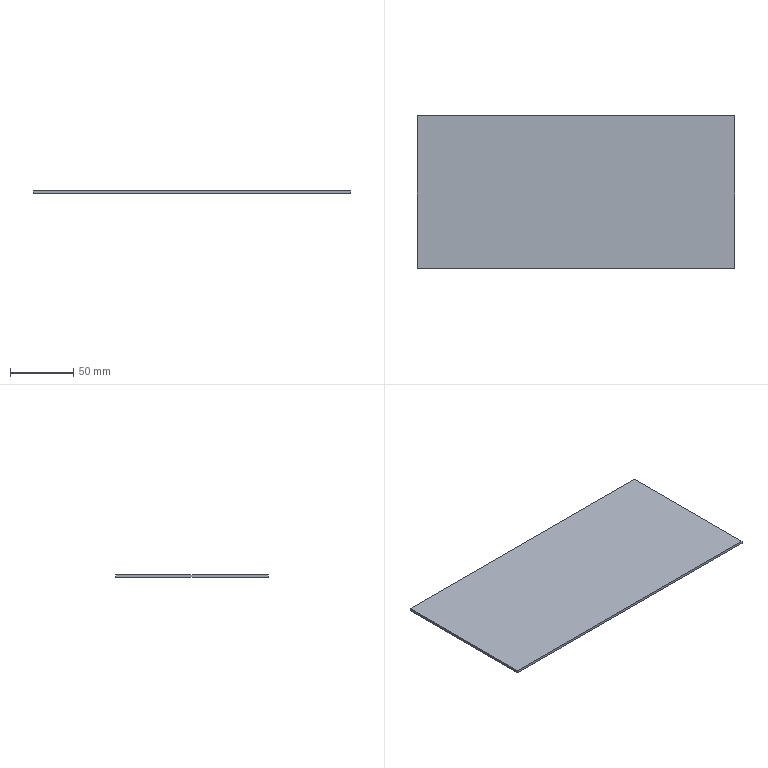Part | SolidWorks | features Extrusion 1 | 1 solid | 6 faces | box 250 x 120 x 2 mm | volume 60000 mm3 | plane 6
STEP:
#1=CARTESIAN_POINT('',(0.,120.,0.));
#2=VERTEX_POINT('',#1);
#3=CARTESIAN_POINT('',(0.,0.,0.));
#4=VERTEX_POINT('',#3);
#5=CARTESIAN_POINT('',(0.,0.,0.));
#6=DIRECTION('',(0.,-1.,0.));
#7=VECTOR('',#6,1000.);
#8=LINE('',#5,#7);
#9=EDGE_CURVE('',#2,#4,#8,.T.);
#10=ORIENTED_EDGE('',*,*,#9,.T.);
#11=CARTESIAN_POINT('',(0.,0.,2.));
#12=VERTEX_POINT('',#11);
#13=CARTESIAN_POINT('',(0.,0.,2.));
#14=DIRECTION('',(0.,0.,-1.));
#15=VECTOR('',#14,1000.);
#16=LINE('',#13,#15);
#17=EDGE_CURVE('',#12,#4,#16,.T.);
#18=ORIENTED_EDGE('',*,*,#17,.F.);
#19=CARTESIAN_POINT('',(0.,120.,2.));
#20=VERTEX_POINT('',#19);
#21=CARTESIAN_POINT('',(0.,0.,2.));
#22=DIRECTION('',(0.,-1.,0.));
#23=VECTOR('',#22,1000.);
#24=LINE('',#21,#23);
#25=EDGE_CURVE('',#20,#12,#24,.T.);
#26=ORIENTED_EDGE('',*,*,#25,.F.);
#27=CARTESIAN_POINT('',(0.,120.,2.));
#28=DIRECTION('',(0.,0.,-1.));
#29=VECTOR('',#28,1000.);
#30=LINE('',#27,#29);
#31=EDGE_CURVE('',#20,#2,#30,.T.);
#32=ORIENTED_EDGE('',*,*,#31,.T.);
#33=EDGE_LOOP('',(#10,#18,#26,#32));
#34=FACE_OUTER_BOUND('',#33,.T.);
#35=CARTESIAN_POINT('',(0.,0.,2.));
#36=DIRECTION('',(1.,0.,0.));
#37=DIRECTION('',(0.,0.,-1.));
#38=AXIS2_PLACEMENT_3D('',#35,#36,#37);
#39=PLANE('',#38);
#40=ADVANCED_FACE('',(#34),#39,.F.);
#41=CARTESIAN_POINT('',(250.,0.,0.));
#42=VERTEX_POINT('',#41);
#43=CARTESIAN_POINT('',(0.,0.,0.));
#44=DIRECTION('',(1.,0.,0.));
#45=VECTOR('',#44,1000.);
#46=LINE('',#43,#45);
#47=EDGE_CURVE('',#4,#42,#46,.T.);
#48=ORIENTED_EDGE('',*,*,#47,.T.);
#49=CARTESIAN_POINT('',(250.,0.,2.));
#50=VERTEX_POINT('',#49);
#51=CARTESIAN_POINT('',(250.,0.,2.));
#52=DIRECTION('',(0.,0.,-1.));
#53=VECTOR('',#52,1000.);
#54=LINE('',#51,#53);
#55=EDGE_CURVE('',#50,#42,#54,.T.);
#56=ORIENTED_EDGE('',*,*,#55,.F.);
#57=CARTESIAN_POINT('',(0.,0.,2.));
#58=DIRECTION('',(1.,0.,0.));
#59=VECTOR('',#58,1000.);
#60=LINE('',#57,#59);
#61=EDGE_CURVE('',#12,#50,#60,.T.);
#62=ORIENTED_EDGE('',*,*,#61,.F.);
#63=ORIENTED_EDGE('',*,*,#17,.T.);
#64=EDGE_LOOP('',(#48,#56,#62,#63));
#65=FACE_OUTER_BOUND('',#64,.T.);
#66=CARTESIAN_POINT('',(0.,0.,2.));
#67=DIRECTION('',(0.,1.,0.));
#68=DIRECTION('',(0.,0.,1.));
#69=AXIS2_PLACEMENT_3D('',#66,#67,#68);
#70=PLANE('',#69);
#71=ADVANCED_FACE('',(#65),#70,.F.);
#72=CARTESIAN_POINT('',(250.,120.,0.));
#73=VERTEX_POINT('',#72);
#74=CARTESIAN_POINT('',(250.,0.,0.));
#75=DIRECTION('',(0.,1.,0.));
#76=VECTOR('',#75,1000.);
#77=LINE('',#74,#76);
#78=EDGE_CURVE('',#42,#73,#77,.T.);
#79=ORIENTED_EDGE('',*,*,#78,.T.);
#80=CARTESIAN_POINT('',(250.,120.,2.));
#81=VERTEX_POINT('',#80);
#82=CARTESIAN_POINT('',(250.,120.,2.));
#83=DIRECTION('',(0.,0.,-1.));
#84=VECTOR('',#83,1000.);
#85=LINE('',#82,#84);
#86=EDGE_CURVE('',#81,#73,#85,.T.);
#87=ORIENTED_EDGE('',*,*,#86,.F.);
#88=CARTESIAN_POINT('',(250.,0.,2.));
#89=DIRECTION('',(0.,1.,0.));
#90=VECTOR('',#89,1000.);
#91=LINE('',#88,#90);
#92=EDGE_CURVE('',#50,#81,#91,.T.);
#93=ORIENTED_EDGE('',*,*,#92,.F.);
#94=ORIENTED_EDGE('',*,*,#55,.T.);
#95=EDGE_LOOP('',(#79,#87,#93,#94));
#96=FACE_OUTER_BOUND('',#95,.T.);
#97=CARTESIAN_POINT('',(250.,0.,2.));
#98=DIRECTION('',(-1.,0.,0.));
#99=DIRECTION('',(0.,0.,1.));
#100=AXIS2_PLACEMENT_3D('',#97,#98,#99);
#101=PLANE('',#100);
#102=ADVANCED_FACE('',(#96),#101,.F.);
#103=CARTESIAN_POINT('',(0.,120.,0.));
#104=DIRECTION('',(-1.,0.,0.));
#105=VECTOR('',#104,1000.);
#106=LINE('',#103,#105);
#107=EDGE_CURVE('',#73,#2,#106,.T.);
#108=ORIENTED_EDGE('',*,*,#107,.T.);
#109=ORIENTED_EDGE('',*,*,#31,.F.);
#110=CARTESIAN_POINT('',(0.,120.,2.));
#111=DIRECTION('',(-1.,0.,0.));
#112=VECTOR('',#111,1000.);
#113=LINE('',#110,#112);
#114=EDGE_CURVE('',#81,#20,#113,.T.);
#115=ORIENTED_EDGE('',*,*,#114,.F.);
#116=ORIENTED_EDGE('',*,*,#86,.T.);
#117=EDGE_LOOP('',(#108,#109,#115,#116));
#118=FACE_OUTER_BOUND('',#117,.T.);
#119=CARTESIAN_POINT('',(0.,120.,2.));
#120=DIRECTION('',(0.,-1.,0.));
#121=DIRECTION('',(0.,0.,-1.));
#122=AXIS2_PLACEMENT_3D('',#119,#120,#121);
#123=PLANE('',#122);
#124=ADVANCED_FACE('',(#118),#123,.F.);
#125=ORIENTED_EDGE('',*,*,#25,.T.);
#126=ORIENTED_EDGE('',*,*,#61,.T.);
#127=ORIENTED_EDGE('',*,*,#92,.T.);
#128=ORIENTED_EDGE('',*,*,#114,.T.);
#129=EDGE_LOOP('',(#125,#126,#127,#128));
#130=FACE_OUTER_BOUND('',#129,.T.);
#131=CARTESIAN_POINT('',(0.,120.,2.));
#132=DIRECTION('',(0.,0.,-1.));
#133=DIRECTION('',(-1.,0.,0.));
#134=AXIS2_PLACEMENT_3D('',#131,#132,#133);
#135=PLANE('',#134);
#136=ADVANCED_FACE('',(#130),#135,.F.);
#137=ORIENTED_EDGE('',*,*,#9,.F.);
#138=ORIENTED_EDGE('',*,*,#107,.F.);
#139=ORIENTED_EDGE('',*,*,#78,.F.);
#140=ORIENTED_EDGE('',*,*,#47,.F.);
#141=EDGE_LOOP('',(#137,#138,#139,#140));
#142=FACE_OUTER_BOUND('',#141,.T.);
#143=CARTESIAN_POINT('',(0.,120.,0.));
#144=DIRECTION('',(0.,0.,-1.));
#145=DIRECTION('',(-1.,0.,0.));
#146=AXIS2_PLACEMENT_3D('',#143,#144,#145);
#147=PLANE('',#146);
#148=ADVANCED_FACE('',(#142),#147,.T.);
#149=CLOSED_SHELL('',(#40,#71,#102,#124,#136,#148));
#150=MANIFOLD_SOLID_BREP('',#149);
#151=CARTESIAN_POINT('',(0.,0.,0.));
#152=DIRECTION('',(0.,0.,1.));
#153=DIRECTION('',(1.,0.,0.));
#154=AXIS2_PLACEMENT_3D('',#151,#152,#153);
#155=(LENGTH_UNIT()NAMED_UNIT(*)SI_UNIT(.MILLI.,.METRE.));
#156=UNCERTAINTY_MEASURE_WITH_UNIT(LENGTH_MEASURE(0.00001),#155,'','');
#157=(NAMED_UNIT(*)PLANE_ANGLE_UNIT()SI_UNIT($,.RADIAN.));
#158=(NAMED_UNIT(*)SI_UNIT($,.STERADIAN.)SOLID_ANGLE_UNIT());
#159=(GEOMETRIC_REPRESENTATION_CONTEXT(3)GLOBAL_UNCERTAINTY_ASSIGNED_CONTEXT((#156))GLOBAL_UNIT_ASSIGNED_CONTEXT((#155,#157,#158))REPRESENTATION_CONTEXT('',''));
#160=ADVANCED_BREP_SHAPE_REPRESENTATION('',(#150,#154),#159);